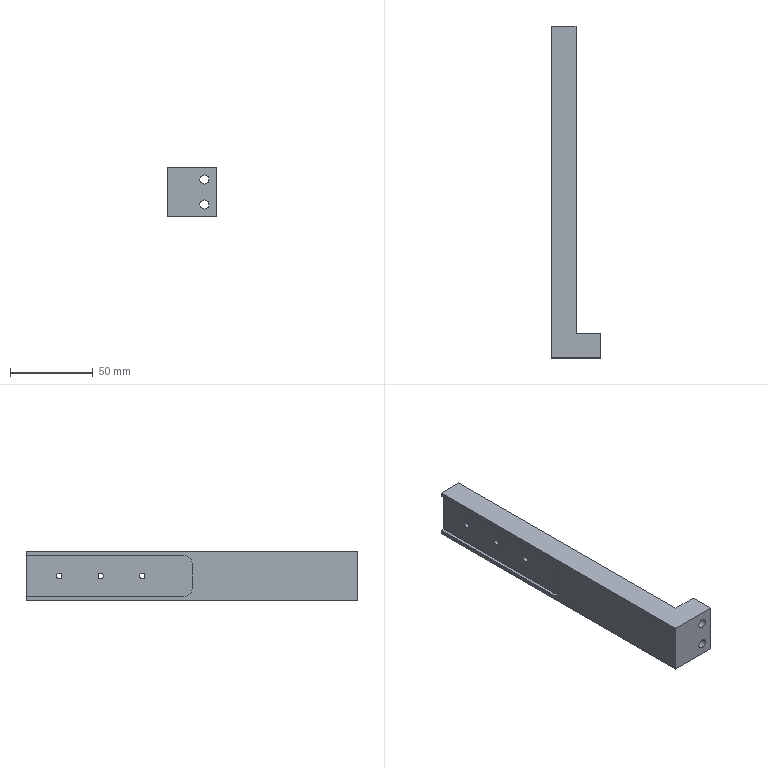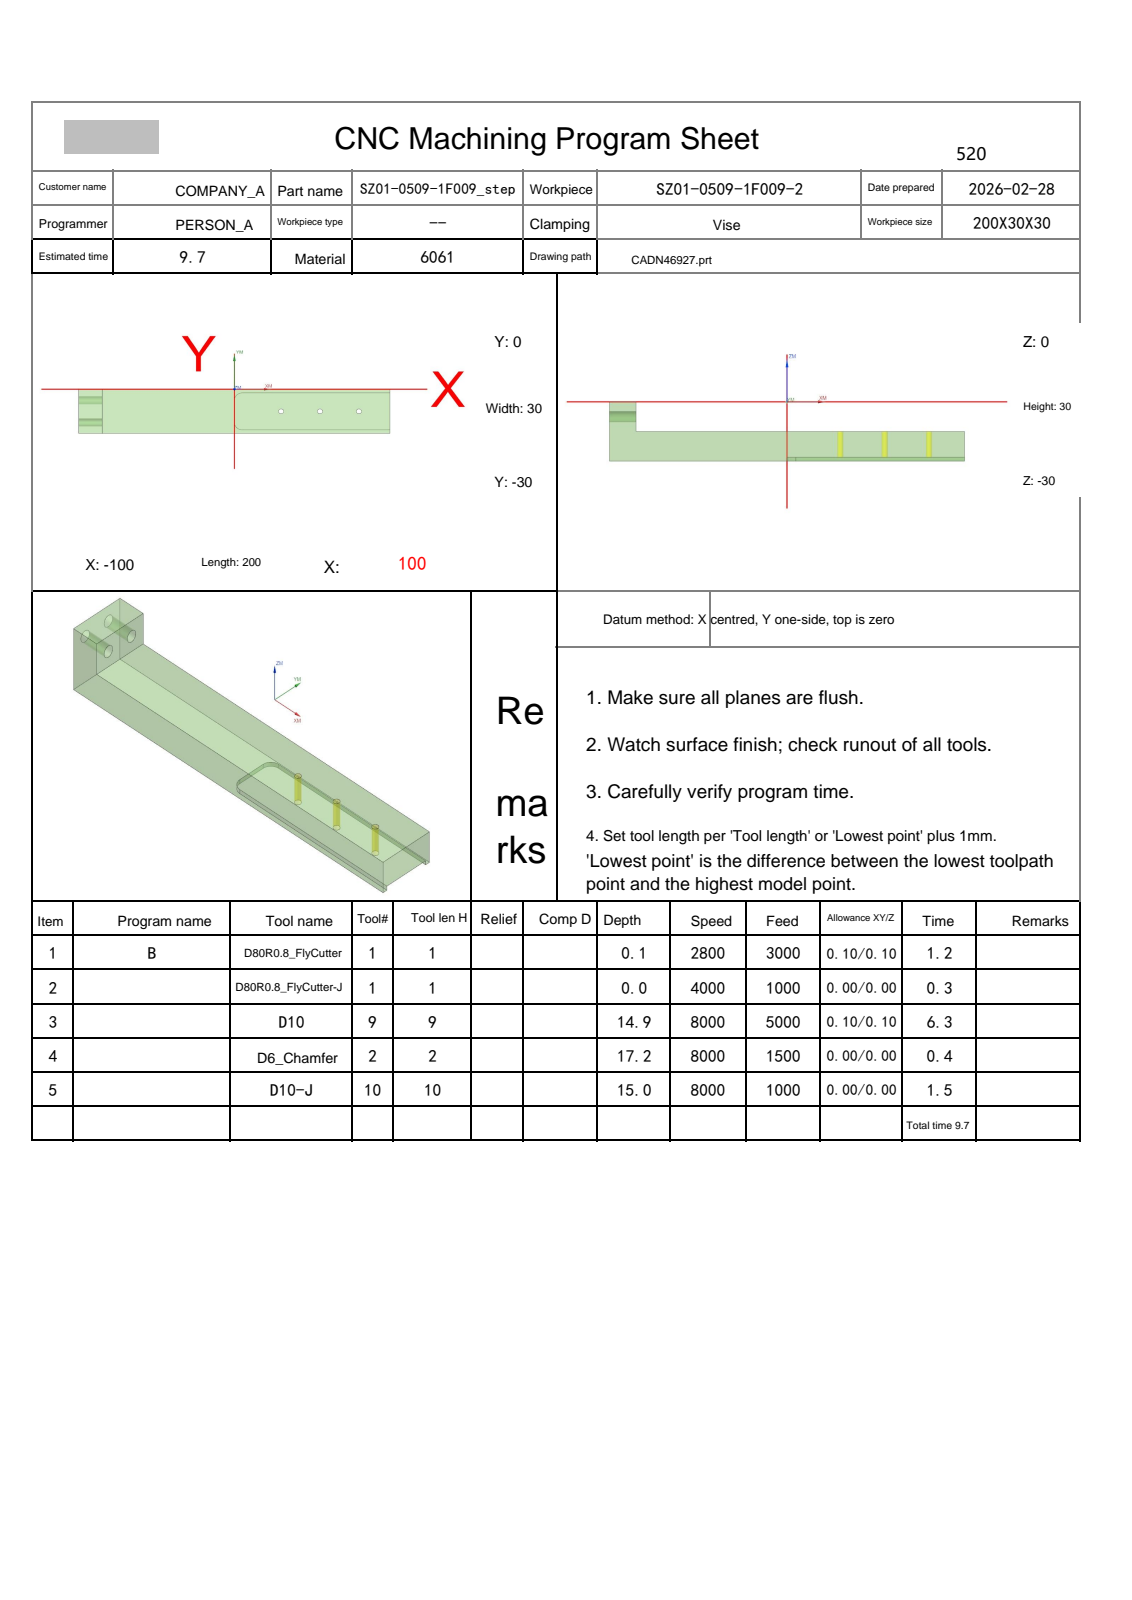NC program | NX | posted by the shop | part box 30 x 200 x 30 mm
Lines 1 to 2718 of 2890, first 1832 of 2716 lines:
%
O0001
(Machine time: 10.59 MIN)
(===Total Tool:4===)
(T1=D80R0.8-FlyCutter D=80.  R=0.8  D-  H01 Z=0.    )
(T9=D10     D=10.  R=0.   D-  H09 Z=-14.9 )
(T2=D6_Chamfer   D=6.   R=0.   D-  H02 Z=-17.2 )
(T10=D10-J  D=10.  R=0.   D10 H10 Z=-15.  )
G80 G90 G17 G49 G40
G91 G28 Z0
M01
N1 T01 M06
(D80R0.8-FlyCutter  D=80. R=0.8 H=01 ce=0.10 di=0.10)
G00 G90 G54 X-152.097 Y-15. M03 S2800
G43 H01 Z50.
M08
Z6.011
G01 Z4.011 F3000.
X-140.097
X140.097
X152.097
Z6.011
G00 X-152.097
Z5.522
G01 Z3.522
X-140.097
X140.097
X152.097
Z5.522
G00 X-152.097
Z5.033
G01 Z3.033
X-140.097
X140.097
X152.097
Z5.033
G00 X-152.097
Z4.544
G01 Z2.544
X-140.097
X140.097
X152.097
Z4.544
G00 Z50.
X-152.097
Z4.056
G01 Z2.056
X-140.097
X140.097
X152.097
Z4.056
G00 Z50.
X-152.097
Z3.567
G01 Z1.567
X-140.097
X140.097
X152.097
Z3.567
G00 Z50.
X-152.097
Z3.078
G01 Z1.078
X-140.097
X140.097
X152.097
Z3.078
G00 Z50.
X-152.097
Z2.589
G01 Z.589
X-140.097
X140.097
X152.097
Z2.589
G00 Z50.
X-152.097
Z2.1
G01 Z.1
X-140.097
X140.097
X152.097
Z2.1
G00 Z50.
G91 G28 Z0.0
M05
M09
G91 G28 Z0.0
M01
N2 T01 M06
(D80R0.8-FlyCutter-J  D=80. R=0.8 H=01 ce=0.00 di=0.00)
G00 G90 G54 X-151.999 Y-15. M03 S4000
G43 H01 Z50.
M08
Z2.
G01 Z0.0 F1000.
X-139.999
X139.999
X151.999
Z2.
G00 Z50.
G91 G28 Z0.0
M05
M09
G91 G28 Z0.0
M01
N3 T09 M06
(D10  D=10. R=0. H=09 ce=0.10 di=0.10)
G00 G90 G54 X100.1 Y8. M03 S8000
G43 H09 Z14.5
M08
Z.904
G01 Z-.596 F5000.
Y4.9
Y-33.901
G02 X99.1 Y-34.9 I-1. J.001
G01 X93.6
G02 X92.6 Y-33.9 I0.0 J1.
G01 Y3.9
G03 X91.6 Y4.9 I-1. J0.0
G01 X86.1
G03 X85.1 Y3.9 I0.0 J-1.
G01 Y-33.9
G02 X84.1 Y-34.9 I-1. J0.0
G01 X78.6
G02 X77.6 Y-33.9 I0.0 J1.
G01 Y3.9
G03 X76.6 Y4.9 I-1. J0.0
G01 X71.1
G03 X70.1 Y3.9 I0.0 J-1.
G01 Y-33.9
G02 X69.1 Y-34.9 I-1. J0.0
G01 X63.6
G02 X62.6 Y-33.9 I0.0 J1.
G01 Y3.901
G03 X61.6 Y4.9 I-1. J-.001
G01 X56.1
G03 X55.1 Y3.9 I0.0 J-1.
G01 Y-33.9
G02 X54.1 Y-34.9 I-1. J0.0
G01 X48.6
G02 X47.6 Y-33.9 I0.0 J1.
G01 Y3.9
G03 X46.6 Y4.9 I-1. J0.0
G01 X41.1
G03 X40.1 Y3.9 I0.0 J-1.
G01 Y-33.9
G02 X39.1 Y-34.9 I-1. J0.0
G01 X33.6
G02 X32.6 Y-33.9 I0.0 J1.
G01 Y3.9
G03 X31.6 Y4.9 I-1. J0.0
G01 X26.1
G03 X25.1 Y3.901 I0.0 J-1.
G01 Y-33.9
G02 X24.1 Y-34.9 I-1. J0.0
G01 X18.6
G02 X17.6 Y-33.9 I0.0 J1.
G01 Y3.9
G03 X16.6 Y4.9 I-1. J0.0
G01 X11.1
G03 X10.1 Y3.9 I0.0 J-1.
G01 Y-33.9
G02 X9.1 Y-34.9 I-1. J0.0
G01 X3.6
G02 X2.6 Y-33.9 I0.0 J1.
G01 Y3.9
G03 X1.6 Y4.9 I-1. J0.0
G01 X-3.9
G03 X-4.9 Y3.9 I0.0 J-1.
G01 Y-33.9
G02 X-5.9 Y-34.9 I-1. J0.0
G01 X-11.4
G02 X-12.4 Y-33.9 I0.0 J1.
G01 Y3.9
G03 X-13.4 Y4.9 I-1. J0.0
G01 X-18.9
G03 X-19.9 Y3.901 I0.0 J-1.
G01 Y-33.9
G02 X-20.899 Y-34.9 I-1. J0.0
G01 X-26.4
G02 X-27.4 Y-33.9 I0.0 J1.
G01 Y3.9
G03 X-28.4 Y4.9 I-1. J0.0
G01 X-33.9
G03 X-34.9 Y3.9 I0.0 J-1.
G01 Y-33.9
G02 X-35.9 Y-34.9 I-1. J0.0
G01 X-41.4
G02 X-42.4 Y-33.9 I0.0 J1.
G01 Y3.9
G03 X-43.4 Y4.9 I-1. J0.0
G01 X-48.9
G03 X-49.9 Y3.9 I0.0 J-1.
G01 Y-33.9
G02 X-50.9 Y-34.9 I-1. J0.0
G01 X-56.4
G02 X-57.4 Y-33.901 I0.0 J1.
G01 Y3.901
G03 X-58.4 Y4.9 I-1. J-.001
G01 X-63.9
G03 X-64.9 Y3.9 I0.0 J-1.
G01 Y-33.901
G02 X-65.9 Y-34.9 I-1. J.001
G01 X-71.4
G02 X-72.4 Y-33.9 I0.0 J1.
G01 Y4.044
G03 X-73.246 Y5.032 I-1. J0.0
G01 X-78.746 Y5.888
X-78.9 Y5.9
G03 X-79.9 Y4.9 I0.0 J-1.
G01 Y-34.9
Y-38.1
Z.904
G00 X100.1 Y8.
Z.308
G01 Z-1.192
Y4.9
Y-33.901
G02 X99.1 Y-34.9 I-1. J.001
G01 X93.6
G02 X92.6 Y-33.9 I0.0 J1.
G01 Y3.9
G03 X91.6 Y4.9 I-1. J0.0
G01 X86.1
G03 X85.1 Y3.9 I0.0 J-1.
G01 Y-33.9
G02 X84.1 Y-34.9 I-1. J0.0
G01 X78.6
G02 X77.6 Y-33.9 I0.0 J1.
G01 Y3.9
G03 X76.6 Y4.9 I-1. J0.0
G01 X71.1
G03 X70.1 Y3.9 I0.0 J-1.
G01 Y-33.9
G02 X69.1 Y-34.9 I-1. J0.0
G01 X63.6
G02 X62.6 Y-33.9 I0.0 J1.
G01 Y3.901
G03 X61.6 Y4.9 I-1. J-.001
G01 X56.1
G03 X55.1 Y3.9 I0.0 J-1.
G01 Y-33.9
G02 X54.1 Y-34.9 I-1. J0.0
G01 X48.6
G02 X47.6 Y-33.9 I0.0 J1.
G01 Y3.9
G03 X46.6 Y4.9 I-1. J0.0
G01 X41.1
G03 X40.1 Y3.9 I0.0 J-1.
G01 Y-33.9
G02 X39.1 Y-34.9 I-1. J0.0
G01 X33.6
G02 X32.6 Y-33.9 I0.0 J1.
G01 Y3.9
G03 X31.6 Y4.9 I-1. J0.0
G01 X26.1
G03 X25.1 Y3.901 I0.0 J-1.
G01 Y-33.9
G02 X24.1 Y-34.9 I-1. J0.0
G01 X18.6
G02 X17.6 Y-33.9 I0.0 J1.
G01 Y3.9
G03 X16.6 Y4.9 I-1. J0.0
G01 X11.1
G03 X10.1 Y3.9 I0.0 J-1.
G01 Y-33.9
G02 X9.1 Y-34.9 I-1. J0.0
G01 X3.6
G02 X2.6 Y-33.9 I0.0 J1.
G01 Y3.9
G03 X1.6 Y4.9 I-1. J0.0
G01 X-3.9
G03 X-4.9 Y3.9 I0.0 J-1.
G01 Y-33.9
G02 X-5.9 Y-34.9 I-1. J0.0
G01 X-11.4
G02 X-12.4 Y-33.9 I0.0 J1.
G01 Y3.9
G03 X-13.4 Y4.9 I-1. J0.0
G01 X-18.9
G03 X-19.9 Y3.901 I0.0 J-1.
G01 Y-33.9
G02 X-20.899 Y-34.9 I-1. J0.0
G01 X-26.4
G02 X-27.4 Y-33.9 I0.0 J1.
G01 Y3.9
G03 X-28.4 Y4.9 I-1. J0.0
G01 X-33.9
G03 X-34.9 Y3.9 I0.0 J-1.
G01 Y-33.9
G02 X-35.9 Y-34.9 I-1. J0.0
G01 X-41.4
G02 X-42.4 Y-33.9 I0.0 J1.
G01 Y3.9
G03 X-43.4 Y4.9 I-1. J0.0
G01 X-48.9
G03 X-49.9 Y3.9 I0.0 J-1.
G01 Y-33.9
G02 X-50.9 Y-34.9 I-1. J0.0
G01 X-56.4
G02 X-57.4 Y-33.901 I0.0 J1.
G01 Y3.901
G03 X-58.4 Y4.9 I-1. J-.001
G01 X-63.9
G03 X-64.9 Y3.9 I0.0 J-1.
G01 Y-33.901
G02 X-65.9 Y-34.9 I-1. J.001
G01 X-71.4
G02 X-72.4 Y-33.9 I0.0 J1.
G01 Y4.044
G03 X-73.246 Y5.032 I-1. J0.0
G01 X-78.746 Y5.888
X-78.9 Y5.9
G03 X-79.9 Y4.9 I0.0 J-1.
G01 Y-34.9
Y-38.1
Z.308
G00 X100.1 Y8.
Z-.288
G01 Z-1.788
Y4.9
Y-33.901
G02 X99.1 Y-34.9 I-1. J.001
G01 X93.6
G02 X92.6 Y-33.9 I0.0 J1.
G01 Y3.9
G03 X91.6 Y4.9 I-1. J0.0
G01 X86.1
G03 X85.1 Y3.9 I0.0 J-1.
G01 Y-33.9
G02 X84.1 Y-34.9 I-1. J0.0
G01 X78.6
G02 X77.6 Y-33.9 I0.0 J1.
G01 Y3.9
G03 X76.6 Y4.9 I-1. J0.0
G01 X71.1
G03 X70.1 Y3.9 I0.0 J-1.
G01 Y-33.9
G02 X69.1 Y-34.9 I-1. J0.0
G01 X63.6
G02 X62.6 Y-33.9 I0.0 J1.
G01 Y3.901
G03 X61.6 Y4.9 I-1. J-.001
G01 X56.1
G03 X55.1 Y3.9 I0.0 J-1.
G01 Y-33.9
G02 X54.1 Y-34.9 I-1. J0.0
G01 X48.6
G02 X47.6 Y-33.9 I0.0 J1.
G01 Y3.9
G03 X46.6 Y4.9 I-1. J0.0
G01 X41.1
G03 X40.1 Y3.9 I0.0 J-1.
G01 Y-33.9
G02 X39.1 Y-34.9 I-1. J0.0
G01 X33.6
G02 X32.6 Y-33.9 I0.0 J1.
G01 Y3.9
G03 X31.6 Y4.9 I-1. J0.0
G01 X26.1
G03 X25.1 Y3.901 I0.0 J-1.
G01 Y-33.9
G02 X24.1 Y-34.9 I-1. J0.0
G01 X18.6
G02 X17.6 Y-33.9 I0.0 J1.
G01 Y3.9
G03 X16.6 Y4.9 I-1. J0.0
G01 X11.1
G03 X10.1 Y3.9 I0.0 J-1.
G01 Y-33.9
G02 X9.1 Y-34.9 I-1. J0.0
G01 X3.6
G02 X2.6 Y-33.9 I0.0 J1.
G01 Y3.9
G03 X1.6 Y4.9 I-1. J0.0
G01 X-3.9
G03 X-4.9 Y3.9 I0.0 J-1.
G01 Y-33.9
G02 X-5.9 Y-34.9 I-1. J0.0
G01 X-11.4
G02 X-12.4 Y-33.9 I0.0 J1.
G01 Y3.9
G03 X-13.4 Y4.9 I-1. J0.0
G01 X-18.9
G03 X-19.9 Y3.901 I0.0 J-1.
G01 Y-33.9
G02 X-20.899 Y-34.9 I-1. J0.0
G01 X-26.4
G02 X-27.4 Y-33.9 I0.0 J1.
G01 Y3.9
G03 X-28.4 Y4.9 I-1. J0.0
G01 X-33.9
G03 X-34.9 Y3.9 I0.0 J-1.
G01 Y-33.9
G02 X-35.9 Y-34.9 I-1. J0.0
G01 X-41.4
G02 X-42.4 Y-33.9 I0.0 J1.
G01 Y3.9
G03 X-43.4 Y4.9 I-1. J0.0
G01 X-48.9
G03 X-49.9 Y3.9 I0.0 J-1.
G01 Y-33.9
G02 X-50.9 Y-34.9 I-1. J0.0
G01 X-56.4
G02 X-57.4 Y-33.901 I0.0 J1.
G01 Y3.901
G03 X-58.4 Y4.9 I-1. J-.001
G01 X-63.9
G03 X-64.9 Y3.9 I0.0 J-1.
G01 Y-33.901
G02 X-65.9 Y-34.9 I-1. J.001
G01 X-71.4
G02 X-72.4 Y-33.9 I0.0 J1.
G01 Y4.044
G03 X-73.246 Y5.032 I-1. J0.0
G01 X-78.746 Y5.888
X-78.9 Y5.9
G03 X-79.9 Y4.9 I0.0 J-1.
G01 Y-34.9
Y-38.1
Z-.288
G00 X100.1 Y8.
Z-.884
G01 Z-2.384
Y4.9
Y-33.901
G02 X99.1 Y-34.9 I-1. J.001
G01 X93.6
G02 X92.6 Y-33.9 I0.0 J1.
G01 Y3.9
G03 X91.6 Y4.9 I-1. J0.0
G01 X86.1
G03 X85.1 Y3.9 I0.0 J-1.
G01 Y-33.9
G02 X84.1 Y-34.9 I-1. J0.0
G01 X78.6
G02 X77.6 Y-33.9 I0.0 J1.
G01 Y3.9
G03 X76.6 Y4.9 I-1. J0.0
G01 X71.1
G03 X70.1 Y3.9 I0.0 J-1.
G01 Y-33.9
G02 X69.1 Y-34.9 I-1. J0.0
G01 X63.6
G02 X62.6 Y-33.9 I0.0 J1.
G01 Y3.901
G03 X61.6 Y4.9 I-1. J-.001
G01 X56.1
G03 X55.1 Y3.9 I0.0 J-1.
G01 Y-33.9
G02 X54.1 Y-34.9 I-1. J0.0
G01 X48.6
G02 X47.6 Y-33.9 I0.0 J1.
G01 Y3.9
G03 X46.6 Y4.9 I-1. J0.0
G01 X41.1
G03 X40.1 Y3.9 I0.0 J-1.
G01 Y-33.9
G02 X39.1 Y-34.9 I-1. J0.0
G01 X33.6
G02 X32.6 Y-33.9 I0.0 J1.
G01 Y3.9
G03 X31.6 Y4.9 I-1. J0.0
G01 X26.1
G03 X25.1 Y3.901 I0.0 J-1.
G01 Y-33.9
G02 X24.1 Y-34.9 I-1. J0.0
G01 X18.6
G02 X17.6 Y-33.9 I0.0 J1.
G01 Y3.9
G03 X16.6 Y4.9 I-1. J0.0
G01 X11.1
G03 X10.1 Y3.9 I0.0 J-1.
G01 Y-33.9
G02 X9.1 Y-34.9 I-1. J0.0
G01 X3.6
G02 X2.6 Y-33.9 I0.0 J1.
G01 Y3.9
G03 X1.6 Y4.9 I-1. J0.0
G01 X-3.9
G03 X-4.9 Y3.9 I0.0 J-1.
G01 Y-33.9
G02 X-5.9 Y-34.9 I-1. J0.0
G01 X-11.4
G02 X-12.4 Y-33.9 I0.0 J1.
G01 Y3.9
G03 X-13.4 Y4.9 I-1. J0.0
G01 X-18.9
G03 X-19.9 Y3.901 I0.0 J-1.
G01 Y-33.9
G02 X-20.899 Y-34.9 I-1. J0.0
G01 X-26.4
G02 X-27.4 Y-33.9 I0.0 J1.
G01 Y3.9
G03 X-28.4 Y4.9 I-1. J0.0
G01 X-33.9
G03 X-34.9 Y3.9 I0.0 J-1.
G01 Y-33.9
G02 X-35.9 Y-34.9 I-1. J0.0
G01 X-41.4
G02 X-42.4 Y-33.9 I0.0 J1.
G01 Y3.9
G03 X-43.4 Y4.9 I-1. J0.0
G01 X-48.9
G03 X-49.9 Y3.9 I0.0 J-1.
G01 Y-33.9
G02 X-50.9 Y-34.9 I-1. J0.0
G01 X-56.4
G02 X-57.4 Y-33.901 I0.0 J1.
G01 Y3.901
G03 X-58.4 Y4.9 I-1. J-.001
G01 X-63.9
G03 X-64.9 Y3.9 I0.0 J-1.
G01 Y-33.901
G02 X-65.9 Y-34.9 I-1. J.001
G01 X-71.4
G02 X-72.4 Y-33.9 I0.0 J1.
G01 Y4.044
G03 X-73.246 Y5.032 I-1. J0.0
G01 X-78.746 Y5.888
X-78.9 Y5.9
G03 X-79.9 Y4.9 I0.0 J-1.
G01 Y-34.9
Y-38.1
Z-.884
G00 X100.1 Y8.
Z-1.48
G01 Z-2.98
Y4.9
Y-33.901
G02 X99.1 Y-34.9 I-1. J.001
G01 X93.6
G02 X92.6 Y-33.9 I0.0 J1.
G01 Y3.9
G03 X91.6 Y4.9 I-1. J0.0
G01 X86.1
G03 X85.1 Y3.9 I0.0 J-1.
G01 Y-33.9
G02 X84.1 Y-34.9 I-1. J0.0
G01 X78.6
G02 X77.6 Y-33.9 I0.0 J1.
G01 Y3.9
G03 X76.6 Y4.9 I-1. J0.0
G01 X71.1
G03 X70.1 Y3.9 I0.0 J-1.
G01 Y-33.9
G02 X69.1 Y-34.9 I-1. J0.0
G01 X63.6
G02 X62.6 Y-33.9 I0.0 J1.
G01 Y3.901
G03 X61.6 Y4.9 I-1. J-.001
G01 X56.1
G03 X55.1 Y3.9 I0.0 J-1.
G01 Y-33.9
G02 X54.1 Y-34.9 I-1. J0.0
G01 X48.6
G02 X47.6 Y-33.9 I0.0 J1.
G01 Y3.9
G03 X46.6 Y4.9 I-1. J0.0
G01 X41.1
G03 X40.1 Y3.9 I0.0 J-1.
G01 Y-33.9
G02 X39.1 Y-34.9 I-1. J0.0
G01 X33.6
G02 X32.6 Y-33.9 I0.0 J1.
G01 Y3.9
G03 X31.6 Y4.9 I-1. J0.0
G01 X26.1
G03 X25.1 Y3.901 I0.0 J-1.
G01 Y-33.9
G02 X24.1 Y-34.9 I-1. J0.0
G01 X18.6
G02 X17.6 Y-33.9 I0.0 J1.
G01 Y3.9
G03 X16.6 Y4.9 I-1. J0.0
G01 X11.1
G03 X10.1 Y3.9 I0.0 J-1.
G01 Y-33.9
G02 X9.1 Y-34.9 I-1. J0.0
G01 X3.6
G02 X2.6 Y-33.9 I0.0 J1.
G01 Y3.9
G03 X1.6 Y4.9 I-1. J0.0
G01 X-3.9
G03 X-4.9 Y3.9 I0.0 J-1.
G01 Y-33.9
G02 X-5.9 Y-34.9 I-1. J0.0
G01 X-11.4
G02 X-12.4 Y-33.9 I0.0 J1.
G01 Y3.9
G03 X-13.4 Y4.9 I-1. J0.0
G01 X-18.9
G03 X-19.9 Y3.901 I0.0 J-1.
G01 Y-33.9
G02 X-20.899 Y-34.9 I-1. J0.0
G01 X-26.4
G02 X-27.4 Y-33.9 I0.0 J1.
G01 Y3.9
G03 X-28.4 Y4.9 I-1. J0.0
G01 X-33.9
G03 X-34.9 Y3.9 I0.0 J-1.
G01 Y-33.9
G02 X-35.9 Y-34.9 I-1. J0.0
G01 X-41.4
G02 X-42.4 Y-33.9 I0.0 J1.
G01 Y3.9
G03 X-43.4 Y4.9 I-1. J0.0
G01 X-48.9
G03 X-49.9 Y3.9 I0.0 J-1.
G01 Y-33.9
G02 X-50.9 Y-34.9 I-1. J0.0
G01 X-56.4
G02 X-57.4 Y-33.901 I0.0 J1.
G01 Y3.901
G03 X-58.4 Y4.9 I-1. J-.001
G01 X-63.9
G03 X-64.9 Y3.9 I0.0 J-1.
G01 Y-33.901
G02 X-65.9 Y-34.9 I-1. J.001
G01 X-71.4
G02 X-72.4 Y-33.9 I0.0 J1.
G01 Y4.044
G03 X-73.246 Y5.032 I-1. J0.0
G01 X-78.746 Y5.888
X-78.9 Y5.9
G03 X-79.9 Y4.9 I0.0 J-1.
G01 Y-34.9
Y-38.1
Z-1.48
G00 X100.1 Y8.
Z-2.076
G01 Z-3.576
Y4.9
Y-33.901
G02 X99.1 Y-34.9 I-1. J.001
G01 X93.6
G02 X92.6 Y-33.9 I0.0 J1.
G01 Y3.9
G03 X91.6 Y4.9 I-1. J0.0
G01 X86.1
G03 X85.1 Y3.9 I0.0 J-1.
G01 Y-33.9
G02 X84.1 Y-34.9 I-1. J0.0
G01 X78.6
G02 X77.6 Y-33.9 I0.0 J1.
G01 Y3.9
G03 X76.6 Y4.9 I-1. J0.0
G01 X71.1
G03 X70.1 Y3.9 I0.0 J-1.
G01 Y-33.9
G02 X69.1 Y-34.9 I-1. J0.0
G01 X63.6
G02 X62.6 Y-33.9 I0.0 J1.
G01 Y3.901
G03 X61.6 Y4.9 I-1. J-.001
G01 X56.1
G03 X55.1 Y3.9 I0.0 J-1.
G01 Y-33.9
G02 X54.1 Y-34.9 I-1. J0.0
G01 X48.6
G02 X47.6 Y-33.9 I0.0 J1.
G01 Y3.9
G03 X46.6 Y4.9 I-1. J0.0
G01 X41.1
G03 X40.1 Y3.9 I0.0 J-1.
G01 Y-33.9
G02 X39.1 Y-34.9 I-1. J0.0
G01 X33.6
G02 X32.6 Y-33.9 I0.0 J1.
G01 Y3.9
G03 X31.6 Y4.9 I-1. J0.0
G01 X26.1
G03 X25.1 Y3.901 I0.0 J-1.
G01 Y-33.9
G02 X24.1 Y-34.9 I-1. J0.0
G01 X18.6
G02 X17.6 Y-33.9 I0.0 J1.
G01 Y3.9
G03 X16.6 Y4.9 I-1. J0.0
G01 X11.1
G03 X10.1 Y3.9 I0.0 J-1.
G01 Y-33.9
G02 X9.1 Y-34.9 I-1. J0.0
G01 X3.6
G02 X2.6 Y-33.9 I0.0 J1.
G01 Y3.9
G03 X1.6 Y4.9 I-1. J0.0
G01 X-3.9
G03 X-4.9 Y3.9 I0.0 J-1.
G01 Y-33.9
G02 X-5.9 Y-34.9 I-1. J0.0
G01 X-11.4
G02 X-12.4 Y-33.9 I0.0 J1.
G01 Y3.9
G03 X-13.4 Y4.9 I-1. J0.0
G01 X-18.9
G03 X-19.9 Y3.901 I0.0 J-1.
G01 Y-33.9
G02 X-20.899 Y-34.9 I-1. J0.0
G01 X-26.4
G02 X-27.4 Y-33.9 I0.0 J1.
G01 Y3.9
G03 X-28.4 Y4.9 I-1. J0.0
G01 X-33.9
G03 X-34.9 Y3.9 I0.0 J-1.
G01 Y-33.9
G02 X-35.9 Y-34.9 I-1. J0.0
G01 X-41.4
G02 X-42.4 Y-33.9 I0.0 J1.
G01 Y3.9
G03 X-43.4 Y4.9 I-1. J0.0
G01 X-48.9
G03 X-49.9 Y3.9 I0.0 J-1.
G01 Y-33.9
G02 X-50.9 Y-34.9 I-1. J0.0
G01 X-56.4
G02 X-57.4 Y-33.901 I0.0 J1.
G01 Y3.901
G03 X-58.4 Y4.9 I-1. J-.001
G01 X-63.9
G03 X-64.9 Y3.9 I0.0 J-1.
G01 Y-33.901
G02 X-65.9 Y-34.9 I-1. J.001
G01 X-71.4
G02 X-72.4 Y-33.9 I0.0 J1.
G01 Y4.044
G03 X-73.246 Y5.032 I-1. J0.0
G01 X-78.746 Y5.888
X-78.9 Y5.9
G03 X-79.9 Y4.9 I0.0 J-1.
G01 Y-34.9
Y-38.1
Z-2.076
G00 X100.1 Y8.
Z-2.672
G01 Z-4.172
Y4.9
Y-33.901
G02 X99.1 Y-34.9 I-1. J.001
G01 X93.6
G02 X92.6 Y-33.9 I0.0 J1.
G01 Y3.9
G03 X91.6 Y4.9 I-1. J0.0
G01 X86.1
G03 X85.1 Y3.9 I0.0 J-1.
G01 Y-33.9
G02 X84.1 Y-34.9 I-1. J0.0
G01 X78.6
G02 X77.6 Y-33.9 I0.0 J1.
G01 Y3.9
G03 X76.6 Y4.9 I-1. J0.0
G01 X71.1
G03 X70.1 Y3.9 I0.0 J-1.
G01 Y-33.9
G02 X69.1 Y-34.9 I-1. J0.0
G01 X63.6
G02 X62.6 Y-33.9 I0.0 J1.
G01 Y3.901
G03 X61.6 Y4.9 I-1. J-.001
G01 X56.1
G03 X55.1 Y3.9 I0.0 J-1.
G01 Y-33.9
G02 X54.1 Y-34.9 I-1. J0.0
G01 X48.6
G02 X47.6 Y-33.9 I0.0 J1.
G01 Y3.9
G03 X46.6 Y4.9 I-1. J0.0
G01 X41.1
G03 X40.1 Y3.9 I0.0 J-1.
G01 Y-33.9
G02 X39.1 Y-34.9 I-1. J0.0
G01 X33.6
G02 X32.6 Y-33.9 I0.0 J1.
G01 Y3.9
G03 X31.6 Y4.9 I-1. J0.0
G01 X26.1
G03 X25.1 Y3.901 I0.0 J-1.
G01 Y-33.9
G02 X24.1 Y-34.9 I-1. J0.0
G01 X18.6
G02 X17.6 Y-33.9 I0.0 J1.
G01 Y3.9
G03 X16.6 Y4.9 I-1. J0.0
G01 X11.1
G03 X10.1 Y3.9 I0.0 J-1.
G01 Y-33.9
G02 X9.1 Y-34.9 I-1. J0.0
G01 X3.6
G02 X2.6 Y-33.9 I0.0 J1.
G01 Y3.9
G03 X1.6 Y4.9 I-1. J0.0
G01 X-3.9
G03 X-4.9 Y3.9 I0.0 J-1.
G01 Y-33.9
G02 X-5.9 Y-34.9 I-1. J0.0
G01 X-11.4
G02 X-12.4 Y-33.9 I0.0 J1.
G01 Y3.9
G03 X-13.4 Y4.9 I-1. J0.0
G01 X-18.9
G03 X-19.9 Y3.901 I0.0 J-1.
G01 Y-33.9
G02 X-20.899 Y-34.9 I-1. J0.0
G01 X-26.4
G02 X-27.4 Y-33.9 I0.0 J1.
G01 Y3.9
G03 X-28.4 Y4.9 I-1. J0.0
G01 X-33.9
G03 X-34.9 Y3.9 I0.0 J-1.
G01 Y-33.9
G02 X-35.9 Y-34.9 I-1. J0.0
G01 X-41.4
G02 X-42.4 Y-33.9 I0.0 J1.
G01 Y3.9
G03 X-43.4 Y4.9 I-1. J0.0
G01 X-48.9
G03 X-49.9 Y3.9 I0.0 J-1.
G01 Y-33.9
G02 X-50.9 Y-34.9 I-1. J0.0
G01 X-56.4
G02 X-57.4 Y-33.901 I0.0 J1.
G01 Y3.901
G03 X-58.4 Y4.9 I-1. J-.001
G01 X-63.9
G03 X-64.9 Y3.9 I0.0 J-1.
G01 Y-33.901
G02 X-65.9 Y-34.9 I-1. J.001
G01 X-71.4
G02 X-72.4 Y-33.9 I0.0 J1.
G01 Y4.044
G03 X-73.246 Y5.032 I-1. J0.0
G01 X-78.746 Y5.888
X-78.9 Y5.9
G03 X-79.9 Y4.9 I0.0 J-1.
G01 Y-34.9
Y-38.1
Z-2.672
G00 X100.1 Y8.
Z-3.268
G01 Z-4.768
Y4.9
Y-33.901
G02 X99.1 Y-34.9 I-1. J.001
G01 X93.6
G02 X92.6 Y-33.9 I0.0 J1.
G01 Y3.9
G03 X91.6 Y4.9 I-1. J0.0
G01 X86.1
G03 X85.1 Y3.9 I0.0 J-1.
G01 Y-33.9
G02 X84.1 Y-34.9 I-1. J0.0
G01 X78.6
G02 X77.6 Y-33.9 I0.0 J1.
G01 Y3.9
G03 X76.6 Y4.9 I-1. J0.0
G01 X71.1
G03 X70.1 Y3.9 I0.0 J-1.
G01 Y-33.9
G02 X69.1 Y-34.9 I-1. J0.0
G01 X63.6
G02 X62.6 Y-33.9 I0.0 J1.
G01 Y3.901
G03 X61.6 Y4.9 I-1. J-.001
G01 X56.1
G03 X55.1 Y3.9 I0.0 J-1.
G01 Y-33.9
G02 X54.1 Y-34.9 I-1. J0.0
G01 X48.6
G02 X47.6 Y-33.9 I0.0 J1.
G01 Y3.9
G03 X46.6 Y4.9 I-1. J0.0
G01 X41.1
G03 X40.1 Y3.9 I0.0 J-1.
G01 Y-33.9
G02 X39.1 Y-34.9 I-1. J0.0
G01 X33.6
G02 X32.6 Y-33.9 I0.0 J1.
G01 Y3.9
G03 X31.6 Y4.9 I-1. J0.0
G01 X26.1
G03 X25.1 Y3.901 I0.0 J-1.
G01 Y-33.9
G02 X24.1 Y-34.9 I-1. J0.0
G01 X18.6
G02 X17.6 Y-33.9 I0.0 J1.
G01 Y3.9
G03 X16.6 Y4.9 I-1. J0.0
G01 X11.1
G03 X10.1 Y3.9 I0.0 J-1.
G01 Y-33.9
G02 X9.1 Y-34.9 I-1. J0.0
G01 X3.6
G02 X2.6 Y-33.9 I0.0 J1.
G01 Y3.9
G03 X1.6 Y4.9 I-1. J0.0
G01 X-3.9
G03 X-4.9 Y3.9 I0.0 J-1.
G01 Y-33.9
G02 X-5.9 Y-34.9 I-1. J0.0
G01 X-11.4
G02 X-12.4 Y-33.9 I0.0 J1.
G01 Y3.9
G03 X-13.4 Y4.9 I-1. J0.0
G01 X-18.9
G03 X-19.9 Y3.901 I0.0 J-1.
G01 Y-33.9
G02 X-20.899 Y-34.9 I-1. J0.0
G01 X-26.4
G02 X-27.4 Y-33.9 I0.0 J1.
G01 Y3.9
G03 X-28.4 Y4.9 I-1. J0.0
G01 X-33.9
G03 X-34.9 Y3.9 I0.0 J-1.
G01 Y-33.9
G02 X-35.9 Y-34.9 I-1. J0.0
G01 X-41.4
G02 X-42.4 Y-33.9 I0.0 J1.
G01 Y3.9
G03 X-43.4 Y4.9 I-1. J0.0
G01 X-48.9
G03 X-49.9 Y3.9 I0.0 J-1.
G01 Y-33.9
G02 X-50.9 Y-34.9 I-1. J0.0
G01 X-56.4
G02 X-57.4 Y-33.901 I0.0 J1.
G01 Y3.901
G03 X-58.4 Y4.9 I-1. J-.001
G01 X-63.9
G03 X-64.9 Y3.9 I0.0 J-1.
G01 Y-33.901
G02 X-65.9 Y-34.9 I-1. J.001
G01 X-71.4
G02 X-72.4 Y-33.9 I0.0 J1.
G01 Y4.044
G03 X-73.246 Y5.032 I-1. J0.0
G01 X-78.746 Y5.888
X-78.9 Y5.9
G03 X-79.9 Y4.9 I0.0 J-1.
G01 Y-34.9
Y-38.1
Z-3.268
G00 X100.1 Y8.
Z-3.864
G01 Z-5.364
Y4.9
Y-33.901
G02 X99.1 Y-34.9 I-1. J.001
G01 X93.6
G02 X92.6 Y-33.9 I0.0 J1.
G01 Y3.9
G03 X91.6 Y4.9 I-1. J0.0
G01 X86.1
G03 X85.1 Y3.9 I0.0 J-1.
G01 Y-33.9
G02 X84.1 Y-34.9 I-1. J0.0
G01 X78.6
G02 X77.6 Y-33.9 I0.0 J1.
G01 Y3.9
G03 X76.6 Y4.9 I-1. J0.0
G01 X71.1
G03 X70.1 Y3.9 I0.0 J-1.
G01 Y-33.9
G02 X69.1 Y-34.9 I-1. J0.0
G01 X63.6
G02 X62.6 Y-33.9 I0.0 J1.
G01 Y3.901
G03 X61.6 Y4.9 I-1. J-.001
G01 X56.1
G03 X55.1 Y3.9 I0.0 J-1.
G01 Y-33.9
G02 X54.1 Y-34.9 I-1. J0.0
G01 X48.6
G02 X47.6 Y-33.9 I0.0 J1.
G01 Y3.9
G03 X46.6 Y4.9 I-1. J0.0
G01 X41.1
G03 X40.1 Y3.9 I0.0 J-1.
G01 Y-33.9
G02 X39.1 Y-34.9 I-1. J0.0
G01 X33.6
G02 X32.6 Y-33.9 I0.0 J1.
G01 Y3.9
G03 X31.6 Y4.9 I-1. J0.0
G01 X26.1
G03 X25.1 Y3.901 I0.0 J-1.
G01 Y-33.9
G02 X24.1 Y-34.9 I-1. J0.0
G01 X18.6
G02 X17.6 Y-33.9 I0.0 J1.
G01 Y3.9
G03 X16.6 Y4.9 I-1. J0.0
G01 X11.1
G03 X10.1 Y3.9 I0.0 J-1.
G01 Y-33.9
G02 X9.1 Y-34.9 I-1. J0.0
G01 X3.6
G02 X2.6 Y-33.9 I0.0 J1.
G01 Y3.9
G03 X1.6 Y4.9 I-1. J0.0
G01 X-3.9
G03 X-4.9 Y3.9 I0.0 J-1.
G01 Y-33.9
G02 X-5.9 Y-34.9 I-1. J0.0
G01 X-11.4
G02 X-12.4 Y-33.9 I0.0 J1.
G01 Y3.9
G03 X-13.4 Y4.9 I-1. J0.0
G01 X-18.9
G03 X-19.9 Y3.901 I0.0 J-1.
G01 Y-33.9
G02 X-20.899 Y-34.9 I-1. J0.0
G01 X-26.4
G02 X-27.4 Y-33.9 I0.0 J1.
G01 Y3.9
G03 X-28.4 Y4.9 I-1. J0.0
G01 X-33.9
G03 X-34.9 Y3.9 I0.0 J-1.
G01 Y-33.9
G02 X-35.9 Y-34.9 I-1. J0.0
G01 X-41.4
G02 X-42.4 Y-33.9 I0.0 J1.
G01 Y3.9
G03 X-43.4 Y4.9 I-1. J0.0
G01 X-48.9
G03 X-49.9 Y3.9 I0.0 J-1.
G01 Y-33.9
G02 X-50.9 Y-34.9 I-1. J0.0
G01 X-56.4
G02 X-57.4 Y-33.901 I0.0 J1.
G01 Y3.901
G03 X-58.4 Y4.9 I-1. J-.001
G01 X-63.9
G03 X-64.9 Y3.9 I0.0 J-1.
G01 Y-33.901
G02 X-65.9 Y-34.9 I-1. J.001
G01 X-71.4
G02 X-72.4 Y-33.9 I0.0 J1.
G01 Y4.044
G03 X-73.246 Y5.032 I-1. J0.0
G01 X-78.746 Y5.888
X-78.9 Y5.9
G03 X-79.9 Y4.9 I0.0 J-1.
G01 Y-34.9
Y-38.1
Z-3.864
G00 X100.1 Y8.
Z-4.46
G01 Z-5.96
Y4.9
Y-33.901
G02 X99.1 Y-34.9 I-1. J.001
G01 X93.6
G02 X92.6 Y-33.9 I0.0 J1.
G01 Y3.9
G03 X91.6 Y4.9 I-1. J0.0
G01 X86.1
G03 X85.1 Y3.9 I0.0 J-1.
G01 Y-33.9
G02 X84.1 Y-34.9 I-1. J0.0
G01 X78.6
G02 X77.6 Y-33.9 I0.0 J1.
G01 Y3.9
G03 X76.6 Y4.9 I-1. J0.0
G01 X71.1
G03 X70.1 Y3.9 I0.0 J-1.
G01 Y-33.9
G02 X69.1 Y-34.9 I-1. J0.0
G01 X63.6
G02 X62.6 Y-33.9 I0.0 J1.
G01 Y3.901
G03 X61.6 Y4.9 I-1. J-.001
G01 X56.1
G03 X55.1 Y3.9 I0.0 J-1.
G01 Y-33.9
G02 X54.1 Y-34.9 I-1. J0.0
G01 X48.6
G02 X47.6 Y-33.9 I0.0 J1.
G01 Y3.9
G03 X46.6 Y4.9 I-1. J0.0
G01 X41.1
G03 X40.1 Y3.9 I0.0 J-1.
G01 Y-33.9
G02 X39.1 Y-34.9 I-1. J0.0
G01 X33.6
G02 X32.6 Y-33.9 I0.0 J1.
G01 Y3.9
G03 X31.6 Y4.9 I-1. J0.0
G01 X26.1
G03 X25.1 Y3.901 I0.0 J-1.
G01 Y-33.9
G02 X24.1 Y-34.9 I-1. J0.0
G01 X18.6
G02 X17.6 Y-33.9 I0.0 J1.
G01 Y3.9
G03 X16.6 Y4.9 I-1. J0.0
G01 X11.1
G03 X10.1 Y3.9 I0.0 J-1.
G01 Y-33.9
G02 X9.1 Y-34.9 I-1. J0.0
G01 X3.6
G02 X2.6 Y-33.9 I0.0 J1.
G01 Y3.9
G03 X1.6 Y4.9 I-1. J0.0
G01 X-3.9
G03 X-4.9 Y3.9 I0.0 J-1.
G01 Y-33.9
G02 X-5.9 Y-34.9 I-1. J0.0
G01 X-11.4
G02 X-12.4 Y-33.9 I0.0 J1.
G01 Y3.9
G03 X-13.4 Y4.9 I-1. J0.0
G01 X-18.9
G03 X-19.9 Y3.901 I0.0 J-1.
G01 Y-33.9
G02 X-20.899 Y-34.9 I-1. J0.0
G01 X-26.4
G02 X-27.4 Y-33.9 I0.0 J1.
G01 Y3.9
G03 X-28.4 Y4.9 I-1. J0.0
G01 X-33.9
G03 X-34.9 Y3.9 I0.0 J-1.
G01 Y-33.9
G02 X-35.9 Y-34.9 I-1. J0.0
G01 X-41.4
G02 X-42.4 Y-33.9 I0.0 J1.
G01 Y3.9
G03 X-43.4 Y4.9 I-1. J0.0
G01 X-48.9
G03 X-49.9 Y3.9 I0.0 J-1.
G01 Y-33.9
G02 X-50.9 Y-34.9 I-1. J0.0
G01 X-56.4
G02 X-57.4 Y-33.901 I0.0 J1.
G01 Y3.901
G03 X-58.4 Y4.9 I-1. J-.001
G01 X-63.9
G03 X-64.9 Y3.9 I0.0 J-1.
G01 Y-33.901
G02 X-65.9 Y-34.9 I-1. J.001
G01 X-71.4
G02 X-72.4 Y-33.9 I0.0 J1.
G01 Y4.044
G03 X-73.246 Y5.032 I-1. J0.0
G01 X-78.746 Y5.888
X-78.9 Y5.9
G03 X-79.9 Y4.9 I0.0 J-1.
G01 Y-34.9
Y-38.1
Z-4.46
G00 X100.1 Y8.
Z-5.056
G01 Z-6.556
Y4.9
Y-33.901
G02 X99.1 Y-34.9 I-1. J.001
G01 X93.6
G02 X92.6 Y-33.9 I0.0 J1.
G01 Y3.9
G03 X91.6 Y4.9 I-1. J0.0
G01 X86.1
G03 X85.1 Y3.9 I0.0 J-1.
G01 Y-33.9
G02 X84.1 Y-34.9 I-1. J0.0
G01 X78.6
G02 X77.6 Y-33.9 I0.0 J1.
G01 Y3.9
G03 X76.6 Y4.9 I-1. J0.0
G01 X71.1
G03 X70.1 Y3.9 I0.0 J-1.
G01 Y-33.9
G02 X69.1 Y-34.9 I-1. J0.0
G01 X63.6
G02 X62.6 Y-33.9 I0.0 J1.
G01 Y3.901
G03 X61.6 Y4.9 I-1. J-.001
G01 X56.1
G03 X55.1 Y3.9 I0.0 J-1.
G01 Y-33.9
G02 X54.1 Y-34.9 I-1. J0.0
G01 X48.6
G02 X47.6 Y-33.9 I0.0 J1.
G01 Y3.9
G03 X46.6 Y4.9 I-1. J0.0
G01 X41.1
G03 X40.1 Y3.9 I0.0 J-1.
G01 Y-33.9
G02 X39.1 Y-34.9 I-1. J0.0
G01 X33.6
G02 X32.6 Y-33.9 I0.0 J1.
G01 Y3.9
G03 X31.6 Y4.9 I-1. J0.0
G01 X26.1
G03 X25.1 Y3.901 I0.0 J-1.
G01 Y-33.9
G02 X24.1 Y-34.9 I-1. J0.0
G01 X18.6
G02 X17.6 Y-33.9 I0.0 J1.
G01 Y3.9
G03 X16.6 Y4.9 I-1. J0.0
G01 X11.1
G03 X10.1 Y3.9 I0.0 J-1.
G01 Y-33.9
G02 X9.1 Y-34.9 I-1. J0.0
G01 X3.6
G02 X2.6 Y-33.9 I0.0 J1.
G01 Y3.9
G03 X1.6 Y4.9 I-1. J0.0
G01 X-3.9
G03 X-4.9 Y3.9 I0.0 J-1.
G01 Y-33.9
G02 X-5.9 Y-34.9 I-1. J0.0
G01 X-11.4
G02 X-12.4 Y-33.9 I0.0 J1.
G01 Y3.9
G03 X-13.4 Y4.9 I-1. J0.0
G01 X-18.9
G03 X-19.9 Y3.901 I0.0 J-1.
G01 Y-33.9
G02 X-20.899 Y-34.9 I-1. J0.0
G01 X-26.4
G02 X-27.4 Y-33.9 I0.0 J1.
G01 Y3.9
G03 X-28.4 Y4.9 I-1. J0.0
G01 X-33.9
G03 X-34.9 Y3.9 I0.0 J-1.
G01 Y-33.9
G02 X-35.9 Y-34.9 I-1. J0.0
G01 X-41.4
G02 X-42.4 Y-33.9 I0.0 J1.
G01 Y3.9
G03 X-43.4 Y4.9 I-1. J0.0
G01 X-48.9
G03 X-49.9 Y3.9 I0.0 J-1.
G01 Y-33.9
G02 X-50.9 Y-34.9 I-1. J0.0
G01 X-56.4
G02 X-57.4 Y-33.901 I0.0 J1.
G01 Y3.901
G03 X-58.4 Y4.9 I-1. J-.001
G01 X-63.9
G03 X-64.9 Y3.9 I0.0 J-1.
G01 Y-33.901
G02 X-65.9 Y-34.9 I-1. J.001
G01 X-71.4
G02 X-72.4 Y-33.9 I0.0 J1.
G01 Y4.044
G03 X-73.246 Y5.032 I-1. J0.0
G01 X-78.746 Y5.888
X-78.9 Y5.9
G03 X-79.9 Y4.9 I0.0 J-1.
G01 Y-34.9
Y-38.1
Z-5.056
G00 X100.1 Y8.
Z-5.652
G01 Z-7.152
Y4.9
Y-33.901
G02 X99.1 Y-34.9 I-1. J.001
G01 X93.6
G02 X92.6 Y-33.9 I0.0 J1.
G01 Y3.9
G03 X91.6 Y4.9 I-1. J0.0
G01 X86.1
G03 X85.1 Y3.9 I0.0 J-1.
G01 Y-33.9
G02 X84.1 Y-34.9 I-1. J0.0
G01 X78.6
G02 X77.6 Y-33.9 I0.0 J1.
G01 Y3.9
G03 X76.6 Y4.9 I-1. J0.0
G01 X71.1
G03 X70.1 Y3.9 I0.0 J-1.
G01 Y-33.9
G02 X69.1 Y-34.9 I-1. J0.0
G01 X63.6
G02 X62.6 Y-33.9 I0.0 J1.
G01 Y3.901
G03 X61.6 Y4.9 I-1. J-.001
G01 X56.1
G03 X55.1 Y3.9 I0.0 J-1.
G01 Y-33.9
G02 X54.1 Y-34.9 I-1. J0.0
G01 X48.6
G02 X47.6 Y-33.9 I0.0 J1.
G01 Y3.9
G03 X46.6 Y4.9 I-1. J0.0
G01 X41.1
G03 X40.1 Y3.9 I0.0 J-1.
G01 Y-33.9
G02 X39.1 Y-34.9 I-1. J0.0
G01 X33.6
G02 X32.6 Y-33.9 I0.0 J1.
G01 Y3.9
G03 X31.6 Y4.9 I-1. J0.0
G01 X26.1
G03 X25.1 Y3.901 I0.0 J-1.
G01 Y-33.9
G02 X24.1 Y-34.9 I-1. J0.0
G01 X18.6
G02 X17.6 Y-33.9 I0.0 J1.
G01 Y3.9
G03 X16.6 Y4.9 I-1. J0.0
G01 X11.1
G03 X10.1 Y3.9 I0.0 J-1.
G01 Y-33.9
G02 X9.1 Y-34.9 I-1. J0.0
G01 X3.6
G02 X2.6 Y-33.9 I0.0 J1.
G01 Y3.9
G03 X1.6 Y4.9 I-1. J0.0
G01 X-3.9
G03 X-4.9 Y3.9 I0.0 J-1.
G01 Y-33.9
G02 X-5.9 Y-34.9 I-1. J0.0
G01 X-11.4
G02 X-12.4 Y-33.9 I0.0 J1.
G01 Y3.9
G03 X-13.4 Y4.9 I-1. J0.0
G01 X-18.9
G03 X-19.9 Y3.901 I0.0 J-1.
G01 Y-33.9
G02 X-20.899 Y-34.9 I-1. J0.0
G01 X-26.4
G02 X-27.4 Y-33.9 I0.0 J1.
G01 Y3.9
G03 X-28.4 Y4.9 I-1. J0.0
G01 X-33.9
G03 X-34.9 Y3.9 I0.0 J-1.
G01 Y-33.9
G02 X-35.9 Y-34.9 I-1. J0.0
G01 X-41.4
G02 X-42.4 Y-33.9 I0.0 J1.
G01 Y3.9
G03 X-43.4 Y4.9 I-1. J0.0
G01 X-48.9
G03 X-49.9 Y3.9 I0.0 J-1.
G01 Y-33.9
G02 X-50.9 Y-34.9 I-1. J0.0
G01 X-56.4
G02 X-57.4 Y-33.901 I0.0 J1.
G01 Y3.901
G03 X-58.4 Y4.9 I-1. J-.001
G01 X-63.9
G03 X-64.9 Y3.9 I0.0 J-1.
G01 Y-33.901
G02 X-65.9 Y-34.9 I-1. J.001
G01 X-71.4
G02 X-72.4 Y-33.9 I0.0 J1.
G01 Y4.044
G03 X-73.246 Y5.032 I-1. J0.0
G01 X-78.746 Y5.888
X-78.9 Y5.9
G03 X-79.9 Y4.9 I0.0 J-1.
G01 Y-34.9
Y-38.1
Z-5.652
G00 X100.1 Y8.
Z-6.248
G01 Z-7.748
Y4.9
Y-33.901
G02 X99.1 Y-34.9 I-1. J.001
G01 X93.6
G02 X92.6 Y-33.9 I0.0 J1.
G01 Y3.9
G03 X91.6 Y4.9 I-1. J0.0
G01 X86.1
G03 X85.1 Y3.9 I0.0 J-1.
G01 Y-33.9
G02 X84.1 Y-34.9 I-1. J0.0
G01 X78.6
G02 X77.6 Y-33.9 I0.0 J1.
G01 Y3.9
G03 X76.6 Y4.9 I-1. J0.0
G01 X71.1
G03 X70.1 Y3.9 I0.0 J-1.
G01 Y-33.9
G02 X69.1 Y-34.9 I-1. J0.0
G01 X63.6
G02 X62.6 Y-33.9 I0.0 J1.
G01 Y3.901
G03 X61.6 Y4.9 I-1. J-.001
G01 X56.1
G03 X55.1 Y3.9 I0.0 J-1.
G01 Y-33.9
G02 X54.1 Y-34.9 I-1. J0.0
G01 X48.6
G02 X47.6 Y-33.9 I0.0 J1.
G01 Y3.9
G03 X46.6 Y4.9 I-1. J0.0
G01 X41.1
G03 X40.1 Y3.9 I0.0 J-1.
G01 Y-33.9
G02 X39.1 Y-34.9 I-1. J0.0
G01 X33.6
G02 X32.6 Y-33.9 I0.0 J1.
G01 Y3.9
G03 X31.6 Y4.9 I-1. J0.0
G01 X26.1
G03 X25.1 Y3.901 I0.0 J-1.
G01 Y-33.9
G02 X24.1 Y-34.9 I-1. J0.0
G01 X18.6
G02 X17.6 Y-33.9 I0.0 J1.
G01 Y3.9
G03 X16.6 Y4.9 I-1. J0.0
G01 X11.1
G03 X10.1 Y3.9 I0.0 J-1.
G01 Y-33.9
G02 X9.1 Y-34.9 I-1. J0.0
G01 X3.6
G02 X2.6 Y-33.9 I0.0 J1.
G01 Y3.9
G03 X1.6 Y4.9 I-1. J0.0
G01 X-3.9
G03 X-4.9 Y3.9 I0.0 J-1.
G01 Y-33.9
G02 X-5.9 Y-34.9 I-1. J0.0
G01 X-11.4
G02 X-12.4 Y-33.9 I0.0 J1.
G01 Y3.9
G03 X-13.4 Y4.9 I-1. J0.0
G01 X-18.9
G03 X-19.9 Y3.901 I0.0 J-1.
G01 Y-33.9
G02 X-20.899 Y-34.9 I-1. J0.0
G01 X-26.4
G02 X-27.4 Y-33.9 I0.0 J1.
G01 Y3.9
G03 X-28.4 Y4.9 I-1. J0.0
G01 X-33.9
G03 X-34.9 Y3.9 I0.0 J-1.
G01 Y-33.9
G02 X-35.9 Y-34.9 I-1. J0.0
G01 X-41.4
G02 X-42.4 Y-33.9 I0.0 J1.
G01 Y3.9
G03 X-43.4 Y4.9 I-1. J0.0
G01 X-48.9
G03 X-49.9 Y3.9 I0.0 J-1.
G01 Y-33.9
G02 X-50.9 Y-34.9 I-1. J0.0
G01 X-56.4
G02 X-57.4 Y-33.901 I0.0 J1.
G01 Y3.901
G03 X-58.4 Y4.9 I-1. J-.001
G01 X-63.9
G03 X-64.9 Y3.9 I0.0 J-1.
G01 Y-33.901
G02 X-65.9 Y-34.9 I-1. J.001
G01 X-71.4
G02 X-72.4 Y-33.9 I0.0 J1.
G01 Y4.044
G03 X-73.246 Y5.032 I-1. J0.0
G01 X-78.746 Y5.888
X-78.9 Y5.9
G03 X-79.9 Y4.9 I0.0 J-1.
G01 Y-34.9
Y-38.1
Z-6.248
G00 X100.1 Y8.
Z-6.844
G01 Z-8.344
Y4.9
Y-33.901
G02 X99.1 Y-34.9 I-1. J.001
G01 X93.6
G02 X92.6 Y-33.9 I0.0 J1.
G01 Y3.9
G03 X91.6 Y4.9 I-1. J0.0
G01 X86.1
G03 X85.1 Y3.9 I0.0 J-1.
G01 Y-33.9
G02 X84.1 Y-34.9 I-1. J0.0
G01 X78.6
G02 X77.6 Y-33.9 I0.0 J1.
G01 Y3.9
G03 X76.6 Y4.9 I-1. J0.0
G01 X71.1
G03 X70.1 Y3.9 I0.0 J-1.
G01 Y-33.9
G02 X69.1 Y-34.9 I-1. J0.0
G01 X63.6
G02 X62.6 Y-33.9 I0.0 J1.
G01 Y3.901
G03 X61.6 Y4.9 I-1. J-.001
G01 X56.1
G03 X55.1 Y3.9 I0.0 J-1.
G01 Y-33.9
G02 X54.1 Y-34.9 I-1. J0.0
G01 X48.6
G02 X47.6 Y-33.9 I0.0 J1.
G01 Y3.9
G03 X46.6 Y4.9 I-1. J0.0
G01 X41.1
G03 X40.1 Y3.9 I0.0 J-1.
G01 Y-33.9
G02 X39.1 Y-34.9 I-1. J0.0
G01 X33.6
G02 X32.6 Y-33.9 I0.0 J1.
G01 Y3.9
G03 X31.6 Y4.9 I-1. J0.0
G01 X26.1
G03 X25.1 Y3.901 I0.0 J-1.
G01 Y-33.9
G02 X24.1 Y-34.9 I-1. J0.0
G01 X18.6
G02 X17.6 Y-33.9 I0.0 J1.
G01 Y3.9
G03 X16.6 Y4.9 I-1. J0.0
G01 X11.1
G03 X10.1 Y3.9 I0.0 J-1.
G01 Y-33.9
G02 X9.1 Y-34.9 I-1. J0.0
G01 X3.6
G02 X2.6 Y-33.9 I0.0 J1.
G01 Y3.9
G03 X1.6 Y4.9 I-1. J0.0
G01 X-3.9
G03 X-4.9 Y3.9 I0.0 J-1.
G01 Y-33.9
G02 X-5.9 Y-34.9 I-1. J0.0
G01 X-11.4
G02 X-12.4 Y-33.9 I0.0 J1.
G01 Y3.9
G03 X-13.4 Y4.9 I-1. J0.0
G01 X-18.9
G03 X-19.9 Y3.901 I0.0 J-1.
G01 Y-33.9
G02 X-20.899 Y-34.9 I-1. J0.0
G01 X-26.4
G02 X-27.4 Y-33.9 I0.0 J1.
G01 Y3.9
G03 X-28.4 Y4.9 I-1. J0.0
G01 X-33.9
G03 X-34.9 Y3.9 I0.0 J-1.
G01 Y-33.9
G02 X-35.9 Y-34.9 I-1. J0.0
G01 X-41.4
G02 X-42.4 Y-33.9 I0.0 J1.
G01 Y3.9
G03 X-43.4 Y4.9 I-1. J0.0
G01 X-48.9
G03 X-49.9 Y3.9 I0.0 J-1.
G01 Y-33.9
G02 X-50.9 Y-34.9 I-1. J0.0
G01 X-56.4
G02 X-57.4 Y-33.901 I0.0 J1.
G01 Y3.901
G03 X-58.4 Y4.9 I-1. J-.001
G01 X-63.9
G03 X-64.9 Y3.9 I0.0 J-1.
G01 Y-33.901
G02 X-65.9 Y-34.9 I-1. J.001
G01 X-71.4
G02 X-72.4 Y-33.9 I0.0 J1.
G01 Y4.044
G03 X-73.246 Y5.032 I-1. J0.0
G01 X-78.746 Y5.888
X-78.9 Y5.9
G03 X-79.9 Y4.9 I0.0 J-1.
G01 Y-34.9
Y-38.1
Z-6.844
G00 X100.1 Y8.
Z-7.44
G01 Z-8.94
Y4.9
Y-33.901
G02 X99.1 Y-34.9 I-1. J.001
G01 X93.6
G02 X92.6 Y-33.9 I0.0 J1.
G01 Y3.9
G03 X91.6 Y4.9 I-1. J0.0
G01 X86.1
G03 X85.1 Y3.9 I0.0 J-1.
G01 Y-33.9
G02 X84.1 Y-34.9 I-1. J0.0
G01 X78.6
G02 X77.6 Y-33.9 I0.0 J1.
G01 Y3.9
G03 X76.6 Y4.9 I-1. J0.0
G01 X71.1
G03 X70.1 Y3.9 I0.0 J-1.
G01 Y-33.9
G02 X69.1 Y-34.9 I-1. J0.0
G01 X63.6
G02 X62.6 Y-33.9 I0.0 J1.
G01 Y3.901
G03 X61.6 Y4.9 I-1. J-.001
G01 X56.1
G03 X55.1 Y3.9 I0.0 J-1.
G01 Y-33.9
G02 X54.1 Y-34.9 I-1. J0.0
G01 X48.6
G02 X47.6 Y-33.9 I0.0 J1.
G01 Y3.9
G03 X46.6 Y4.9 I-1. J0.0
G01 X41.1
G03 X40.1 Y3.9 I0.0 J-1.
G01 Y-33.9
G02 X39.1 Y-34.9 I-1. J0.0
G01 X33.6
G02 X32.6 Y-33.9 I0.0 J1.
G01 Y3.9
G03 X31.6 Y4.9 I-1. J0.0
G01 X26.1
G03 X25.1 Y3.901 I0.0 J-1.
G01 Y-33.9
G02 X24.1 Y-34.9 I-1. J0.0
G01 X18.6
G02 X17.6 Y-33.9 I0.0 J1.
G01 Y3.9
G03 X16.6 Y4.9 I-1. J0.0
G01 X11.1
G03 X10.1 Y3.9 I0.0 J-1.
G01 Y-33.9
G02 X9.1 Y-34.9 I-1. J0.0
G01 X3.6
G02 X2.6 Y-33.9 I0.0 J1.
G01 Y3.9
G03 X1.6 Y4.9 I-1. J0.0
G01 X-3.9
G03 X-4.9 Y3.9 I0.0 J-1.
G01 Y-33.9
G02 X-5.9 Y-34.9 I-1. J0.0
G01 X-11.4
G02 X-12.4 Y-33.9 I0.0 J1.
G01 Y3.9
G03 X-13.4 Y4.9 I-1. J0.0
G01 X-18.9
G03 X-19.9 Y3.901 I0.0 J-1.
G01 Y-33.9
G02 X-20.899 Y-34.9 I-1. J0.0
G01 X-26.4
G02 X-27.4 Y-33.9 I0.0 J1.
G01 Y3.9
G03 X-28.4 Y4.9 I-1. J0.0
G01 X-33.9
G03 X-34.9 Y3.9 I0.0 J-1.
G01 Y-33.9
G02 X-35.9 Y-34.9 I-1. J0.0
G01 X-41.4
G02 X-42.4 Y-33.9 I0.0 J1.
G01 Y3.9
G03 X-43.4 Y4.9 I-1. J0.0
G01 X-48.9
G03 X-49.9 Y3.9 I0.0 J-1.
G01 Y-33.9
G02 X-50.9 Y-34.9 I-1. J0.0
G01 X-56.4
G02 X-57.4 Y-33.901 I0.0 J1.
G01 Y3.901
G03 X-58.4 Y4.9 I-1. J-.001
G01 X-63.9
G03 X-64.9 Y3.9 I0.0 J-1.
G01 Y-33.901
G02 X-65.9 Y-34.9 I-1. J.001
G01 X-71.4
G02 X-72.4 Y-33.9 I0.0 J1.
G01 Y4.044
G03 X-73.246 Y5.032 I-1. J0.0
G01 X-78.746 Y5.888
X-78.9 Y5.9
G03 X-79.9 Y4.9 I0.0 J-1.
G01 Y-34.9
Y-38.1
Z-7.44
G00 X100.1 Y8.
Z-8.036
G01 Z-9.536
Y4.9
Y-33.901
G02 X99.1 Y-34.9 I-1. J.001
G01 X93.6
G02 X92.6 Y-33.9 I0.0 J1.
G01 Y3.9
G03 X91.6 Y4.9 I-1. J0.0
G01 X86.1
G03 X85.1 Y3.9 I0.0 J-1.
G01 Y-33.9
G02 X84.1 Y-34.9 I-1. J0.0
G01 X78.6
G02 X77.6 Y-33.9 I0.0 J1.
G01 Y3.9
G03 X76.6 Y4.9 I-1. J0.0
G01 X71.1
G03 X70.1 Y3.9 I0.0 J-1.
G01 Y-33.9
G02 X69.1 Y-34.9 I-1. J0.0
G01 X63.6
G02 X62.6 Y-33.9 I0.0 J1.
G01 Y3.901
G03 X61.6 Y4.9 I-1. J-.001
G01 X56.1
G03 X55.1 Y3.9 I0.0 J-1.
G01 Y-33.9
G02 X54.1 Y-34.9 I-1. J0.0
G01 X48.6
G02 X47.6 Y-33.9 I0.0 J1.
G01 Y3.9
G03 X46.6 Y4.9 I-1. J0.0
G01 X41.1
G03 X40.1 Y3.9 I0.0 J-1.
G01 Y-33.9
G02 X39.1 Y-34.9 I-1. J0.0
G01 X33.6
G02 X32.6 Y-33.9 I0.0 J1.
G01 Y3.9
G03 X31.6 Y4.9 I-1. J0.0
G01 X26.1
G03 X25.1 Y3.901 I0.0 J-1.
G01 Y-33.9
G02 X24.1 Y-34.9 I-1. J0.0
G01 X18.6
G02 X17.6 Y-33.9 I0.0 J1.
G01 Y3.9
G03 X16.6 Y4.9 I-1. J0.0
G01 X11.1
G03 X10.1 Y3.9 I0.0 J-1.
G01 Y-33.9
G02 X9.1 Y-34.9 I-1. J0.0
G01 X3.6
G02 X2.6 Y-33.9 I0.0 J1.
G01 Y3.9
G03 X1.6 Y4.9 I-1. J0.0
G01 X-3.9
G03 X-4.9 Y3.9 I0.0 J-1.
G01 Y-33.9
G02 X-5.9 Y-34.9 I-1. J0.0
G01 X-11.4
G02 X-12.4 Y-33.9 I0.0 J1.
G01 Y3.9
G03 X-13.4 Y4.9 I-1. J0.0
G01 X-18.9
G03 X-19.9 Y3.901 I0.0 J-1.
G01 Y-33.9
G02 X-20.899 Y-34.9 I-1. J0.0
G01 X-26.4
G02 X-27.4 Y-33.9 I0.0 J1.
G01 Y3.9
G03 X-28.4 Y4.9 I-1. J0.0
G01 X-33.9
G03 X-34.9 Y3.9 I0.0 J-1.
G01 Y-33.9
G02 X-35.9 Y-34.9 I-1. J0.0
G01 X-41.4
G02 X-42.4 Y-33.9 I0.0 J1.
G01 Y3.9
G03 X-43.4 Y4.9 I-1. J0.0
G01 X-48.9
G03 X-49.9 Y3.9 I0.0 J-1.
G01 Y-33.9
G02 X-50.9 Y-34.9 I-1. J0.0
G01 X-56.4
G02 X-57.4 Y-33.901 I0.0 J1.
G01 Y3.901
G03 X-58.4 Y4.9 I-1. J-.001
G01 X-63.9
G03 X-64.9 Y3.9 I0.0 J-1.
G01 Y-33.901
G02 X-65.9 Y-34.9 I-1. J.001
G01 X-71.4
G02 X-72.4 Y-33.9 I0.0 J1.
G01 Y4.044
G03 X-73.246 Y5.032 I-1. J0.0
G01 X-78.746 Y5.888
X-78.9 Y5.9
G03 X-79.9 Y4.9 I0.0 J-1.
G01 Y-34.9
Y-38.1
Z-8.036
G00 X100.1 Y8.
Z-8.632
G01 Z-10.132
Y4.9
Y-33.901
G02 X99.1 Y-34.9 I-1. J.001
G01 X93.6
G02 X92.6 Y-33.9 I0.0 J1.
G01 Y3.9
G03 X91.6 Y4.9 I-1. J0.0
G01 X86.1
G03 X85.1 Y3.9 I0.0 J-1.
G01 Y-33.9
G02 X84.1 Y-34.9 I-1. J0.0
G01 X78.6
G02 X77.6 Y-33.9 I0.0 J1.
G01 Y3.9
G03 X76.6 Y4.9 I-1. J0.0
G01 X71.1
G03 X70.1 Y3.9 I0.0 J-1.
G01 Y-33.9
G02 X69.1 Y-34.9 I-1. J0.0
G01 X63.6
G02 X62.6 Y-33.9 I0.0 J1.
G01 Y3.901
G03 X61.6 Y4.9 I-1. J-.001
G01 X56.1
G03 X55.1 Y3.9 I0.0 J-1.
G01 Y-33.9
G02 X54.1 Y-34.9 I-1. J0.0
G01 X48.6
G02 X47.6 Y-33.9 I0.0 J1.
G01 Y3.9
G03 X46.6 Y4.9 I-1. J0.0
G01 X41.1
G03 X40.1 Y3.9 I0.0 J-1.
G01 Y-33.9
G02 X39.1 Y-34.9 I-1. J0.0
G01 X33.6
G02 X32.6 Y-33.9 I0.0 J1.
G01 Y3.9
G03 X31.6 Y4.9 I-1. J0.0
G01 X26.1
G03 X25.1 Y3.901 I0.0 J-1.
G01 Y-33.9
G02 X24.1 Y-34.9 I-1. J0.0
G01 X18.6
G02 X17.6 Y-33.9 I0.0 J1.
G01 Y3.9
G03 X16.6 Y4.9 I-1. J0.0
G01 X11.1
G03 X10.1 Y3.9 I0.0 J-1.
G01 Y-33.9
G02 X9.1 Y-34.9 I-1. J0.0
G01 X3.6
G02 X2.6 Y-33.9 I0.0 J1.
G01 Y3.9
G03 X1.6 Y4.9 I-1. J0.0